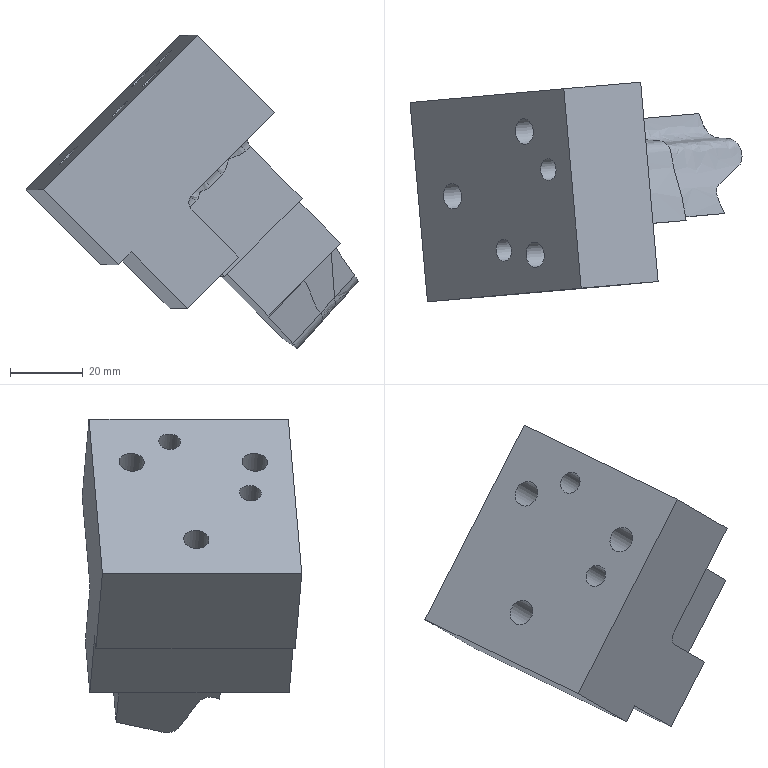Part | NX | features solid 2 | 1 solid | 58 faces | box 91.254 x 60.337 x 86.158 mm | volume 141612 mm3 | spline 23 | plane 21 | cylinder 14 | commonest cylinder face diameters 6 x8 7 x3 11 x3